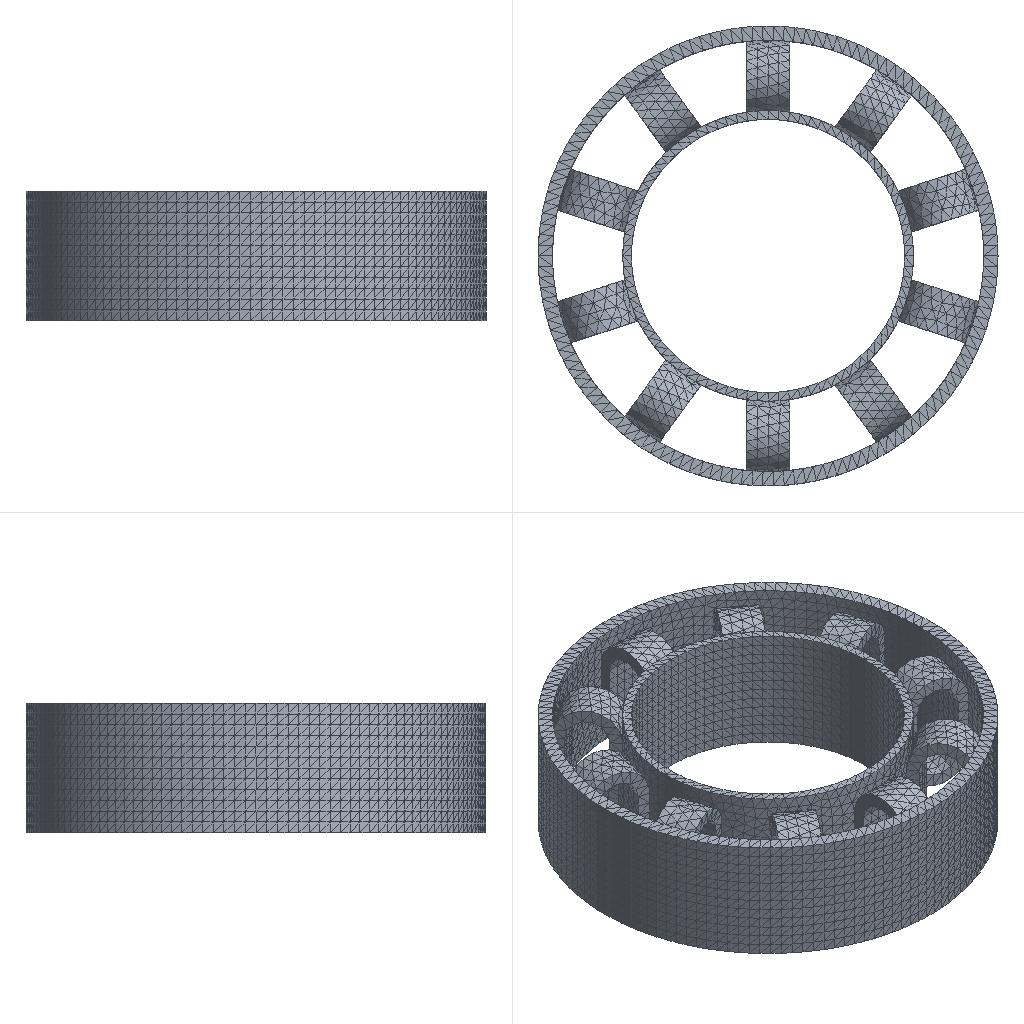Simulation study | abaqus
Set-up summary:
category,name,step,type,value,unit,region
solver,abaqus
solver,version,,,Abaqus/Standard 3DEXPERIENCE R2017x
units,not stated in the deck,,not stated
analysis,deck,,transient,transient
load_step,Step-1,Step-1,transient
load_step,requested,,,1
mesh,nodes,,,11472
mesh,elements,,,38959
element_type,R3D4,,rigid,528
element_type,C3D4H,,solid,38431
load,load commands in deck,,count,2
bc,support commands in deck,,count,11
material,MATERIAL-1,,in results
check,setup vs results,,match,"per instance, exact: element labels, types and connectivity; labels of the nodes the elements use; coordinates of those nodes at SINGLE_PRECISION in 1 of 2 instance(s)"
Abaqus input file, long lists of numbers shortened:
*Heading
** Job name: Job-1 Model name: Model-1
** Generated by: Abaqus/CAE 2017
*Preprint, echo=NO, model=NO, history=NO, contact=NO
**
** PARTS
**
*Part, name=road
*Node
      1,         240.,           0.,           0.
      2,         225.,           0.,           0.
** (576 more lines like these left out)
*Element, type=R3D4
  1,   1,   2,  19,  18
  2,   2,   3,  20,  19
** (526 more lines like these left out)
*Node
    579,         240.,        -500.,           0.
*Nset, nset=road-RefPt_, internal
579,
*Elset, elset=road, generate
   1,  528,    1
*End Part
**
*Part, name=work
*Node
      1,  -209.088,  -49.011,         -40.
      2,  -197.964,  -83.249,         -40.
** (10891 more lines like these left out)
*Element, type=C3D4H
   1,   20, 9385,  446, 3615
   2, 9385,  445,    8,  388
** (38429 more lines like these left out)
*Nset, nset=Set-5, generate
     1,  10893,      1
*Elset, elset=Set-5, generate
     1,  38431,      1
** Section: Section-1
*Solid Section, elset=Set-5, material=Material-1
,
*End Part
**
**
** ASSEMBLY
**
*Assembly, name=Assembly
**
*Instance, name=work-1, part=work
*End Instance
**
*Instance, name=road-1, part=road
       -320.,         250.,        -120.
       -320.,         250.,        -120.,        -320.,         249.,        -120.,          90.
*End Instance
**
*Node
      1,           0.,           0.,           0.
*Nset, nset=Set-2
 1,
*Nset, nset=Set-3, instance=road-1
 579,
*Nset, nset=Set-4, instance=road-1
 579,
*Nset, nset=Set-5, instance=work-1, generate
     1,  10893,      1
*Elset, elset=Set-5, instance=work-1, generate
     1,  38431,      1
*Nset, nset=Set-6
 1,
*Nset, nset=m_Set-1
 1,
*Elset, elset=_m_Surf-2_SNEG, internal, instance=road-1, generate
   1,  528,    1
*Surface, type=ELEMENT, name=m_Surf-2
_m_Surf-2_SNEG, SNEG
*Elset, elset=_s_Surf-1_S1, internal, instance=work-1
 13857, 14008, 14014, 14037, 14044, 14057, 14066, 14082, 14088, 14213, 14254, 14305, 14455, 14469, 14549, 14589
 14592, 14610, 14660, 14698, 14738, 14740, 14748, 14753, 14779, 14799, 14811, 14834, 14873, 14892, 14893, 14936
** (19 more lines like these left out)
*Elset, elset=_s_Surf-1_S3, internal, instance=work-1
 13864, 13877, 13885, 13902, 13906, 13913, 13916, 13926, 13931, 13949, 13951, 13975, 13979, 13990, 14003, 14010
 14022, 14032, 14034, 14052, 14060, 14063, 14095, 14099, 14131, 14152, 14161, 14184, 14196, 14211, 14221, 14239
** (45 more lines like these left out)
*Elset, elset=_s_Surf-1_S2, internal, instance=work-1
 13888, 14002, 14007, 14026, 14031, 14047, 14058, 14073, 14078, 14084, 14098, 14122, 14124, 14146, 14156, 14181
 14204, 14244, 14319, 14339, 14409, 14618, 14640, 14664, 14683, 14702, 14726, 14747, 14764, 14810, 14826, 14843
** (23 more lines like these left out)
*Elset, elset=_s_Surf-1_S4, internal, instance=work-1
 14001, 14009, 14013, 14017, 14029, 14049, 14061, 14070, 14072, 14077, 14079, 14087, 14092, 14094, 14103, 14140
 14145, 14159, 14160, 14165, 14182, 14215, 14276, 14288, 14294, 14335, 14377, 14383, 14400, 14430, 14462, 14468
** (32 more lines like these left out)
*Surface, type=ELEMENT, name=s_Surf-1
_s_Surf-1_S1, S1
_s_Surf-1_S3, S3
_s_Surf-1_S2, S2
_s_Surf-1_S4, S4
*Elset, elset=_s_Surf-2_S3, internal, instance=work-1
 20458, 20527, 20588, 20691, 20894, 20915, 20941, 21024, 21114, 21154, 21182, 21302, 21321, 21361, 21428, 21436
 21445, 21474, 21509, 21573, 21574, 21629, 21636, 21683, 21751, 21753, 21787, 21816, 21821, 21847, 21864, 21956
** (195 more lines like these left out)
*Elset, elset=_s_Surf-2_S1, internal, instance=work-1
 24704, 25493, 25649, 27264, 28763, 29760, 30210, 32454, 34783, 35142
*Elset, elset=_s_Surf-2_S2, internal, instance=work-1
 20515, 20528, 20747, 23905, 25458, 25534, 25619, 25654, 25661, 26012, 26239, 26315, 27561, 28192, 28805, 30003
 30330, 32315, 32341, 33842, 33895, 34157, 34640, 36504, 37773
*Elset, elset=_s_Surf-2_S4, internal, instance=work-1
 20541, 21060, 21391, 22961, 24192, 24485, 24638, 24645, 25097, 25711, 25766, 26211, 26577, 27094, 27351, 27646
 27798, 28641, 28737, 28792, 29119, 30699, 31176, 31613, 32466, 32723, 33377, 33503, 33590, 33652, 33872, 33947
** (1 more lines like these left out)
*Surface, type=ELEMENT, name=s_Surf-2
_s_Surf-2_S3, S3
_s_Surf-2_S1, S1
_s_Surf-2_S2, S2
_s_Surf-2_S4, S4
*Rigid Body, ref node=road-1.road-RefPt_, elset=road-1.road
** Constraint: Constraint-1
*Coupling, constraint name=Constraint-1, ref node=m_Set-1, surface=s_Surf-1
*Kinematic
*End Assembly
*Amplitude, name=Amp-1
             0.,              0.,              5.,              1.
**
** MATERIALS
**
*Material, name=Material-1
*Conductivity
 0.214,
*Density
 1.2e-09,
*Expansion
 0.001,
*Hyperelastic, n=3, ogden
 -5.75,  3.36, 0.017,  6.42, 16.17, -6.12,    0.,    0.
    0.,
*Specific Heat
 2.37e+09,
**
** INTERACTION PROPERTIES
**
*Surface Interaction, name=IntProp-1
1.,
*Friction
0.,
*Surface Behavior, pressure-overclosure=HARD
**
** INTERACTIONS
**
** Interaction: Int-1
*Contact Pair, interaction=IntProp-1, type=SURFACE TO SURFACE, adjust=0.5
s_Surf-2, m_Surf-2
** ----------------------------------------------------------------
**
** STEP: Step-1
**
*Step, name=Step-1, nlgeom=YES, inc=1000
*Dynamic
0.01,5.,5e-05
**
** BOUNDARY CONDITIONS
**
** Name: BC-3 Type: 位移/转角
*Boundary, amplitude=Amp-1
Set-6, 1, 1
Set-6, 2, 2
Set-6, 3, 3
Set-6, 4, 4
Set-6, 5, 5
Set-6, 6, 6, 12.
** Name: [REDACTED] : Displacement/rotation angle
*Boundary
Set-4, 2, 2
Set-4, 3, 3
Set-4, 4, 4
Set-4, 5, 5
Set-4, 6, 6
**
** LOADS
**
** Name: Load-1   Type: Concentrated force
*Cload
Set-3, 1, 1000.
**
** PREDEFINED FIELDS
**
** Name: Predefined Field-1   Type: Temperature
*Temperature, file=D:\________________\_____\_____.______________________________________
**
** OUTPUT REQUESTS
**
*Restart, write, frequency=0
**
** FIELD OUTPUT: F-Output-1
**
*Output, field, frequency=1
*Node Output
CF, NT, RF, RM, RT, U, V
*Element Output, directions=YES
E, FV, LE, MISES, MISESONLY, PE, PEEQ, PEMAG, PRESSONLY, S, SDV, SSAVG, TEMP
*Contact Output
CDISP, CSTRESS
**
** HISTORY OUTPUT: H-Output-1
**
*Output, history, variable=PRESELECT, frequency=1
*End Step
Results summary:
result,step,,completed,increments=146 time=5.0/5.0
result,analysis,,,transient
result,last_loadstep,,,1
result,primary field,,,U
result,reaction total,,FX,-1001.932,model units
result,reaction total,,FY,-1.398,model units
result,reaction total,,FZ,0.05334,model units